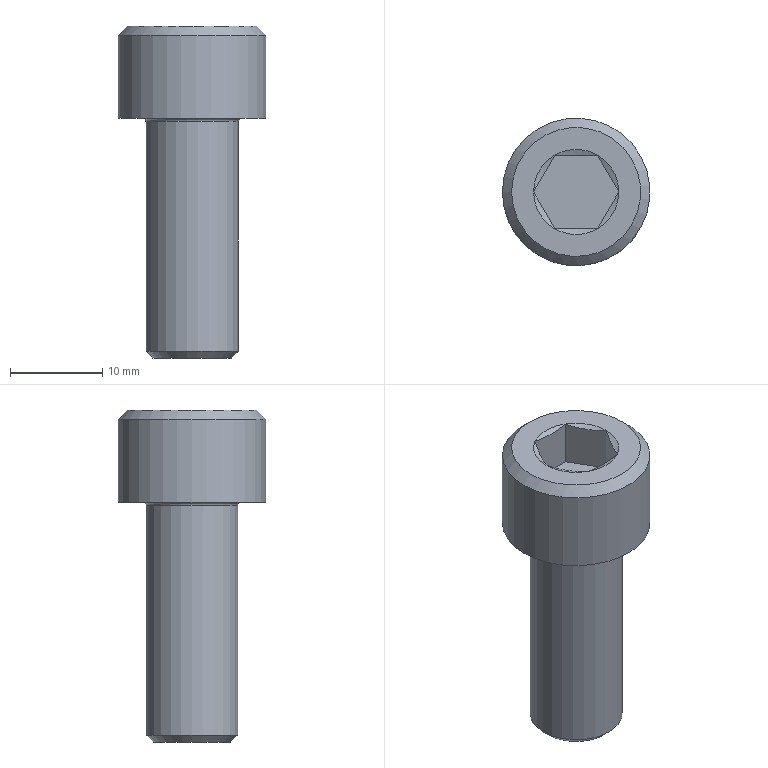Part | STEP file | solid 71 | 1 solid | 21 faces | box 16 x 16 x 36 mm | volume 3743 mm3 | plane 10 | sphere 6 | cylinder 2 | cone 2 | torus 1 | commonest cylinder face diameters 10 x1 16 x1